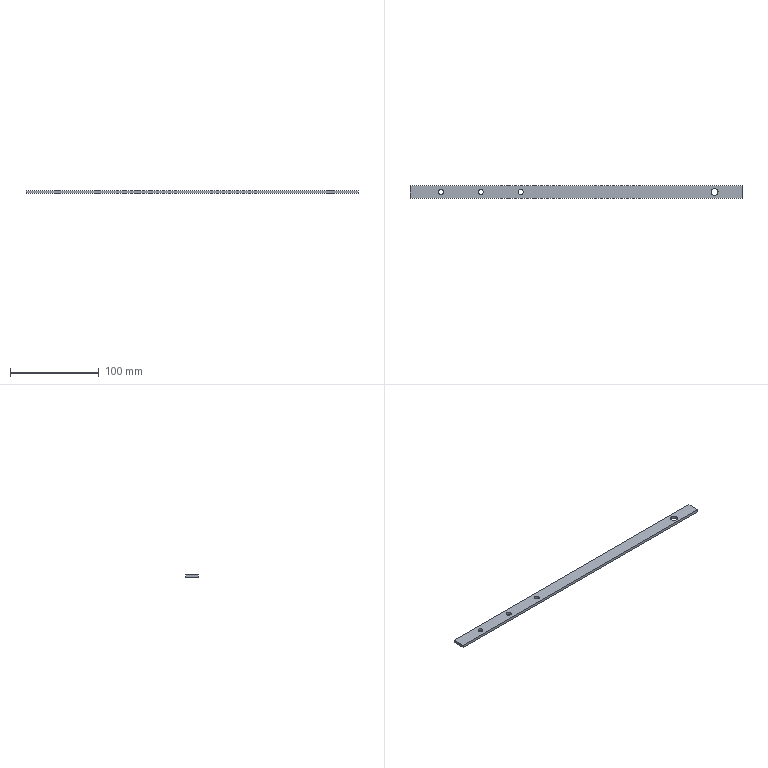Part | SolidWorks | features Extrusion 1, ICE 1 | 1 solid | 14 faces | box 375 x 14 x 3 mm | volume 15385 mm3 | cylinder 8 | plane 6 | commonest cylinder face diameters 5.5 x6 8 x2
STEP:
#1=CARTESIAN_POINT('',(152.5,0.,-1.5));
#2=VERTEX_POINT('',#1);
#3=CARTESIAN_POINT('',(160.5,0.,-1.5));
#4=VERTEX_POINT('',#3);
#5=CARTESIAN_POINT('',(156.5,0.,-1.5));
#6=DIRECTION('',(0.,0.,1.));
#7=DIRECTION('',(1.,0.,0.));
#8=AXIS2_PLACEMENT_3D('',#5,#6,#7);
#9=CIRCLE('',#8,4.);
#10=EDGE_CURVE('',#2,#4,#9,.T.);
#11=ORIENTED_EDGE('',*,*,#10,.F.);
#12=CARTESIAN_POINT('',(152.5,0.,1.5));
#13=VERTEX_POINT('',#12);
#14=CARTESIAN_POINT('',(152.5,0.,-1.5));
#15=DIRECTION('',(0.,0.,1.));
#16=VECTOR('',#15,1000.);
#17=LINE('',#14,#16);
#18=EDGE_CURVE('',#2,#13,#17,.T.);
#19=ORIENTED_EDGE('',*,*,#18,.T.);
#20=CARTESIAN_POINT('',(160.5,0.,1.5));
#21=VERTEX_POINT('',#20);
#22=CARTESIAN_POINT('',(156.5,0.,1.5));
#23=DIRECTION('',(0.,0.,1.));
#24=DIRECTION('',(1.,0.,0.));
#25=AXIS2_PLACEMENT_3D('',#22,#23,#24);
#26=CIRCLE('',#25,4.);
#27=EDGE_CURVE('',#13,#21,#26,.T.);
#28=ORIENTED_EDGE('',*,*,#27,.T.);
#29=CARTESIAN_POINT('',(160.5,0.,-1.5));
#30=DIRECTION('',(0.,0.,1.));
#31=VECTOR('',#30,1000.);
#32=LINE('',#29,#31);
#33=EDGE_CURVE('',#4,#21,#32,.T.);
#34=ORIENTED_EDGE('',*,*,#33,.F.);
#35=EDGE_LOOP('',(#11,#19,#28,#34));
#36=FACE_OUTER_BOUND('',#35,.T.);
#37=CARTESIAN_POINT('',(156.5,0.,-1.5));
#38=DIRECTION('',(0.,0.,1.));
#39=DIRECTION('',(1.,0.,0.));
#40=AXIS2_PLACEMENT_3D('',#37,#38,#39);
#41=CYLINDRICAL_SURFACE('',#40,4.);
#42=ADVANCED_FACE('',(#36),#41,.F.);
#43=CARTESIAN_POINT('',(-65.25,0.,1.5));
#44=VERTEX_POINT('',#43);
#45=CARTESIAN_POINT('',(-59.75,0.,1.5));
#46=VERTEX_POINT('',#45);
#47=CARTESIAN_POINT('',(-62.5,0.,1.5));
#48=DIRECTION('',(0.,0.,1.));
#49=DIRECTION('',(1.,0.,0.));
#50=AXIS2_PLACEMENT_3D('',#47,#48,#49);
#51=CIRCLE('',#50,2.75);
#52=EDGE_CURVE('',#44,#46,#51,.T.);
#53=ORIENTED_EDGE('',*,*,#52,.T.);
#54=CARTESIAN_POINT('',(-59.75,0.,-1.5));
#55=VERTEX_POINT('',#54);
#56=CARTESIAN_POINT('',(-59.75,0.,1.5));
#57=DIRECTION('',(0.,0.,-1.));
#58=VECTOR('',#57,1000.);
#59=LINE('',#56,#58);
#60=EDGE_CURVE('',#46,#55,#59,.T.);
#61=ORIENTED_EDGE('',*,*,#60,.T.);
#62=CARTESIAN_POINT('',(-65.25,0.,-1.5));
#63=VERTEX_POINT('',#62);
#64=CARTESIAN_POINT('',(-62.5,0.,-1.5));
#65=DIRECTION('',(0.,0.,1.));
#66=DIRECTION('',(1.,0.,0.));
#67=AXIS2_PLACEMENT_3D('',#64,#65,#66);
#68=CIRCLE('',#67,2.75);
#69=EDGE_CURVE('',#63,#55,#68,.T.);
#70=ORIENTED_EDGE('',*,*,#69,.F.);
#71=CARTESIAN_POINT('',(-65.25,0.,1.5));
#72=DIRECTION('',(0.,0.,-1.));
#73=VECTOR('',#72,1000.);
#74=LINE('',#71,#73);
#75=EDGE_CURVE('',#44,#63,#74,.T.);
#76=ORIENTED_EDGE('',*,*,#75,.F.);
#77=EDGE_LOOP('',(#53,#61,#70,#76));
#78=FACE_OUTER_BOUND('',#77,.T.);
#79=CARTESIAN_POINT('',(-62.5,0.,1.5));
#80=DIRECTION('',(0.,0.,-1.));
#81=DIRECTION('',(-1.,0.,0.));
#82=AXIS2_PLACEMENT_3D('',#79,#80,#81);
#83=CYLINDRICAL_SURFACE('',#82,2.75);
#84=ADVANCED_FACE('',(#78),#83,.F.);
#85=CARTESIAN_POINT('',(-110.25,0.,1.5));
#86=VERTEX_POINT('',#85);
#87=CARTESIAN_POINT('',(-104.75,0.,1.5));
#88=VERTEX_POINT('',#87);
#89=CARTESIAN_POINT('',(-107.5,0.,1.5));
#90=DIRECTION('',(0.,0.,1.));
#91=DIRECTION('',(1.,0.,0.));
#92=AXIS2_PLACEMENT_3D('',#89,#90,#91);
#93=CIRCLE('',#92,2.75);
#94=EDGE_CURVE('',#86,#88,#93,.T.);
#95=ORIENTED_EDGE('',*,*,#94,.T.);
#96=CARTESIAN_POINT('',(-104.75,0.,-1.5));
#97=VERTEX_POINT('',#96);
#98=CARTESIAN_POINT('',(-104.75,0.,1.5));
#99=DIRECTION('',(0.,0.,-1.));
#100=VECTOR('',#99,1000.);
#101=LINE('',#98,#100);
#102=EDGE_CURVE('',#88,#97,#101,.T.);
#103=ORIENTED_EDGE('',*,*,#102,.T.);
#104=CARTESIAN_POINT('',(-110.25,0.,-1.5));
#105=VERTEX_POINT('',#104);
#106=CARTESIAN_POINT('',(-107.5,0.,-1.5));
#107=DIRECTION('',(0.,0.,1.));
#108=DIRECTION('',(1.,0.,0.));
#109=AXIS2_PLACEMENT_3D('',#106,#107,#108);
#110=CIRCLE('',#109,2.75);
#111=EDGE_CURVE('',#105,#97,#110,.T.);
#112=ORIENTED_EDGE('',*,*,#111,.F.);
#113=CARTESIAN_POINT('',(-110.25,0.,1.5));
#114=DIRECTION('',(0.,0.,-1.));
#115=VECTOR('',#114,1000.);
#116=LINE('',#113,#115);
#117=EDGE_CURVE('',#86,#105,#116,.T.);
#118=ORIENTED_EDGE('',*,*,#117,.F.);
#119=EDGE_LOOP('',(#95,#103,#112,#118));
#120=FACE_OUTER_BOUND('',#119,.T.);
#121=CARTESIAN_POINT('',(-107.5,0.,1.5));
#122=DIRECTION('',(0.,0.,-1.));
#123=DIRECTION('',(-1.,0.,0.));
#124=AXIS2_PLACEMENT_3D('',#121,#122,#123);
#125=CYLINDRICAL_SURFACE('',#124,2.75);
#126=ADVANCED_FACE('',(#120),#125,.F.);
#127=CARTESIAN_POINT('',(-155.25,0.,1.5));
#128=VERTEX_POINT('',#127);
#129=CARTESIAN_POINT('',(-149.75,0.,1.5));
#130=VERTEX_POINT('',#129);
#131=CARTESIAN_POINT('',(-152.5,0.,1.5));
#132=DIRECTION('',(0.,0.,1.));
#133=DIRECTION('',(1.,0.,0.));
#134=AXIS2_PLACEMENT_3D('',#131,#132,#133);
#135=CIRCLE('',#134,2.75);
#136=EDGE_CURVE('',#128,#130,#135,.T.);
#137=ORIENTED_EDGE('',*,*,#136,.T.);
#138=CARTESIAN_POINT('',(-149.75,0.,-1.5));
#139=VERTEX_POINT('',#138);
#140=CARTESIAN_POINT('',(-149.75,0.,1.5));
#141=DIRECTION('',(0.,0.,-1.));
#142=VECTOR('',#141,1000.);
#143=LINE('',#140,#142);
#144=EDGE_CURVE('',#130,#139,#143,.T.);
#145=ORIENTED_EDGE('',*,*,#144,.T.);
#146=CARTESIAN_POINT('',(-155.25,0.,-1.5));
#147=VERTEX_POINT('',#146);
#148=CARTESIAN_POINT('',(-152.5,0.,-1.5));
#149=DIRECTION('',(0.,0.,1.));
#150=DIRECTION('',(1.,0.,0.));
#151=AXIS2_PLACEMENT_3D('',#148,#149,#150);
#152=CIRCLE('',#151,2.75);
#153=EDGE_CURVE('',#147,#139,#152,.T.);
#154=ORIENTED_EDGE('',*,*,#153,.F.);
#155=CARTESIAN_POINT('',(-155.25,0.,1.5));
#156=DIRECTION('',(0.,0.,-1.));
#157=VECTOR('',#156,1000.);
#158=LINE('',#155,#157);
#159=EDGE_CURVE('',#128,#147,#158,.T.);
#160=ORIENTED_EDGE('',*,*,#159,.F.);
#161=EDGE_LOOP('',(#137,#145,#154,#160));
#162=FACE_OUTER_BOUND('',#161,.T.);
#163=CARTESIAN_POINT('',(-152.5,0.,1.5));
#164=DIRECTION('',(0.,0.,-1.));
#165=DIRECTION('',(-1.,0.,0.));
#166=AXIS2_PLACEMENT_3D('',#163,#164,#165);
#167=CYLINDRICAL_SURFACE('',#166,2.75);
#168=ADVANCED_FACE('',(#162),#167,.F.);
#169=CARTESIAN_POINT('',(156.5,0.,1.5));
#170=DIRECTION('',(0.,0.,1.));
#171=DIRECTION('',(1.,0.,0.));
#172=AXIS2_PLACEMENT_3D('',#169,#170,#171);
#173=CIRCLE('',#172,4.);
#174=EDGE_CURVE('',#21,#13,#173,.T.);
#175=ORIENTED_EDGE('',*,*,#174,.F.);
#176=ORIENTED_EDGE('',*,*,#27,.F.);
#177=EDGE_LOOP('',(#175,#176));
#178=FACE_BOUND('',#177,.T.);
#179=ORIENTED_EDGE('',*,*,#94,.F.);
#180=CARTESIAN_POINT('',(-107.5,0.,1.5));
#181=DIRECTION('',(0.,0.,1.));
#182=DIRECTION('',(1.,0.,0.));
#183=AXIS2_PLACEMENT_3D('',#180,#181,#182);
#184=CIRCLE('',#183,2.75);
#185=EDGE_CURVE('',#88,#86,#184,.T.);
#186=ORIENTED_EDGE('',*,*,#185,.F.);
#187=EDGE_LOOP('',(#179,#186));
#188=FACE_BOUND('',#187,.T.);
#189=CARTESIAN_POINT('',(-187.5,7.,1.5));
#190=VERTEX_POINT('',#189);
#191=CARTESIAN_POINT('',(-187.5,-7.,1.5));
#192=VERTEX_POINT('',#191);
#193=CARTESIAN_POINT('',(-187.5,-7.,1.5));
#194=DIRECTION('',(0.,-1.,0.));
#195=VECTOR('',#194,1000.);
#196=LINE('',#193,#195);
#197=EDGE_CURVE('',#190,#192,#196,.T.);
#198=ORIENTED_EDGE('',*,*,#197,.T.);
#199=CARTESIAN_POINT('',(187.5,-7.,1.5));
#200=VERTEX_POINT('',#199);
#201=CARTESIAN_POINT('',(187.5,-7.,1.5));
#202=DIRECTION('',(1.,0.,0.));
#203=VECTOR('',#202,1000.);
#204=LINE('',#201,#203);
#205=EDGE_CURVE('',#192,#200,#204,.T.);
#206=ORIENTED_EDGE('',*,*,#205,.T.);
#207=CARTESIAN_POINT('',(187.5,7.,1.5));
#208=VERTEX_POINT('',#207);
#209=CARTESIAN_POINT('',(187.5,-7.,1.5));
#210=DIRECTION('',(0.,1.,0.));
#211=VECTOR('',#210,1000.);
#212=LINE('',#209,#211);
#213=EDGE_CURVE('',#200,#208,#212,.T.);
#214=ORIENTED_EDGE('',*,*,#213,.T.);
#215=CARTESIAN_POINT('',(187.5,7.,1.5));
#216=DIRECTION('',(-1.,0.,0.));
#217=VECTOR('',#216,1000.);
#218=LINE('',#215,#217);
#219=EDGE_CURVE('',#208,#190,#218,.T.);
#220=ORIENTED_EDGE('',*,*,#219,.T.);
#221=EDGE_LOOP('',(#198,#206,#214,#220));
#222=FACE_OUTER_BOUND('',#221,.T.);
#223=ORIENTED_EDGE('',*,*,#136,.F.);
#224=CARTESIAN_POINT('',(-152.5,0.,1.5));
#225=DIRECTION('',(0.,0.,1.));
#226=DIRECTION('',(1.,0.,0.));
#227=AXIS2_PLACEMENT_3D('',#224,#225,#226);
#228=CIRCLE('',#227,2.75);
#229=EDGE_CURVE('',#130,#128,#228,.T.);
#230=ORIENTED_EDGE('',*,*,#229,.F.);
#231=EDGE_LOOP('',(#223,#230));
#232=FACE_BOUND('',#231,.T.);
#233=ORIENTED_EDGE('',*,*,#52,.F.);
#234=CARTESIAN_POINT('',(-62.5,0.,1.5));
#235=DIRECTION('',(0.,0.,1.));
#236=DIRECTION('',(1.,0.,0.));
#237=AXIS2_PLACEMENT_3D('',#234,#235,#236);
#238=CIRCLE('',#237,2.75);
#239=EDGE_CURVE('',#46,#44,#238,.T.);
#240=ORIENTED_EDGE('',*,*,#239,.F.);
#241=EDGE_LOOP('',(#233,#240));
#242=FACE_BOUND('',#241,.T.);
#243=CARTESIAN_POINT('',(0.,0.,1.5));
#244=DIRECTION('',(0.,0.,1.));
#245=DIRECTION('',(1.,0.,0.));
#246=AXIS2_PLACEMENT_3D('',#243,#244,#245);
#247=PLANE('',#246);
#248=ADVANCED_FACE('',(#178,#188,#222,#232,#242),#247,.T.);
#249=CARTESIAN_POINT('',(156.5,0.,-1.5));
#250=DIRECTION('',(0.,0.,1.));
#251=DIRECTION('',(1.,0.,0.));
#252=AXIS2_PLACEMENT_3D('',#249,#250,#251);
#253=CIRCLE('',#252,4.);
#254=EDGE_CURVE('',#4,#2,#253,.T.);
#255=ORIENTED_EDGE('',*,*,#254,.T.);
#256=ORIENTED_EDGE('',*,*,#10,.T.);
#257=EDGE_LOOP('',(#255,#256));
#258=FACE_BOUND('',#257,.T.);
#259=CARTESIAN_POINT('',(-187.5,7.,-1.5));
#260=VERTEX_POINT('',#259);
#261=CARTESIAN_POINT('',(-187.5,-7.,-1.5));
#262=VERTEX_POINT('',#261);
#263=CARTESIAN_POINT('',(-187.5,-7.,-1.5));
#264=DIRECTION('',(0.,-1.,0.));
#265=VECTOR('',#264,1000.);
#266=LINE('',#263,#265);
#267=EDGE_CURVE('',#260,#262,#266,.T.);
#268=ORIENTED_EDGE('',*,*,#267,.F.);
#269=CARTESIAN_POINT('',(187.5,7.,-1.5));
#270=VERTEX_POINT('',#269);
#271=CARTESIAN_POINT('',(187.5,7.,-1.5));
#272=DIRECTION('',(-1.,0.,0.));
#273=VECTOR('',#272,1000.);
#274=LINE('',#271,#273);
#275=EDGE_CURVE('',#270,#260,#274,.T.);
#276=ORIENTED_EDGE('',*,*,#275,.F.);
#277=CARTESIAN_POINT('',(187.5,-7.,-1.5));
#278=VERTEX_POINT('',#277);
#279=CARTESIAN_POINT('',(187.5,-7.,-1.5));
#280=DIRECTION('',(0.,1.,0.));
#281=VECTOR('',#280,1000.);
#282=LINE('',#279,#281);
#283=EDGE_CURVE('',#278,#270,#282,.T.);
#284=ORIENTED_EDGE('',*,*,#283,.F.);
#285=CARTESIAN_POINT('',(187.5,-7.,-1.5));
#286=DIRECTION('',(1.,0.,0.));
#287=VECTOR('',#286,1000.);
#288=LINE('',#285,#287);
#289=EDGE_CURVE('',#262,#278,#288,.T.);
#290=ORIENTED_EDGE('',*,*,#289,.F.);
#291=EDGE_LOOP('',(#268,#276,#284,#290));
#292=FACE_OUTER_BOUND('',#291,.T.);
#293=ORIENTED_EDGE('',*,*,#153,.T.);
#294=CARTESIAN_POINT('',(-152.5,0.,-1.5));
#295=DIRECTION('',(0.,0.,1.));
#296=DIRECTION('',(1.,0.,0.));
#297=AXIS2_PLACEMENT_3D('',#294,#295,#296);
#298=CIRCLE('',#297,2.75);
#299=EDGE_CURVE('',#139,#147,#298,.T.);
#300=ORIENTED_EDGE('',*,*,#299,.T.);
#301=EDGE_LOOP('',(#293,#300));
#302=FACE_BOUND('',#301,.T.);
#303=ORIENTED_EDGE('',*,*,#111,.T.);
#304=CARTESIAN_POINT('',(-107.5,0.,-1.5));
#305=DIRECTION('',(0.,0.,1.));
#306=DIRECTION('',(1.,0.,0.));
#307=AXIS2_PLACEMENT_3D('',#304,#305,#306);
#308=CIRCLE('',#307,2.75);
#309=EDGE_CURVE('',#97,#105,#308,.T.);
#310=ORIENTED_EDGE('',*,*,#309,.T.);
#311=EDGE_LOOP('',(#303,#310));
#312=FACE_BOUND('',#311,.T.);
#313=ORIENTED_EDGE('',*,*,#69,.T.);
#314=CARTESIAN_POINT('',(-62.5,0.,-1.5));
#315=DIRECTION('',(0.,0.,1.));
#316=DIRECTION('',(1.,0.,0.));
#317=AXIS2_PLACEMENT_3D('',#314,#315,#316);
#318=CIRCLE('',#317,2.75);
#319=EDGE_CURVE('',#55,#63,#318,.T.);
#320=ORIENTED_EDGE('',*,*,#319,.T.);
#321=EDGE_LOOP('',(#313,#320));
#322=FACE_BOUND('',#321,.T.);
#323=CARTESIAN_POINT('',(0.,0.,-1.5));
#324=DIRECTION('',(0.,0.,1.));
#325=DIRECTION('',(1.,0.,0.));
#326=AXIS2_PLACEMENT_3D('',#323,#324,#325);
#327=PLANE('',#326);
#328=ADVANCED_FACE('',(#258,#292,#302,#312,#322),#327,.F.);
#329=ORIENTED_EDGE('',*,*,#267,.T.);
#330=CARTESIAN_POINT('',(-187.5,-7.,1.5));
#331=DIRECTION('',(0.,0.,-1.));
#332=VECTOR('',#331,1000.);
#333=LINE('',#330,#332);
#334=EDGE_CURVE('',#192,#262,#333,.T.);
#335=ORIENTED_EDGE('',*,*,#334,.F.);
#336=ORIENTED_EDGE('',*,*,#197,.F.);
#337=CARTESIAN_POINT('',(-187.5,7.,1.5));
#338=DIRECTION('',(0.,0.,-1.));
#339=VECTOR('',#338,1000.);
#340=LINE('',#337,#339);
#341=EDGE_CURVE('',#190,#260,#340,.T.);
#342=ORIENTED_EDGE('',*,*,#341,.T.);
#343=EDGE_LOOP('',(#329,#335,#336,#342));
#344=FACE_OUTER_BOUND('',#343,.T.);
#345=CARTESIAN_POINT('',(-187.5,-7.,1.5));
#346=DIRECTION('',(1.,0.,0.));
#347=DIRECTION('',(0.,0.,-1.));
#348=AXIS2_PLACEMENT_3D('',#345,#346,#347);
#349=PLANE('',#348);
#350=ADVANCED_FACE('',(#344),#349,.F.);
#351=ORIENTED_EDGE('',*,*,#289,.T.);
#352=CARTESIAN_POINT('',(187.5,-7.,1.5));
#353=DIRECTION('',(0.,0.,-1.));
#354=VECTOR('',#353,1000.);
#355=LINE('',#352,#354);
#356=EDGE_CURVE('',#200,#278,#355,.T.);
#357=ORIENTED_EDGE('',*,*,#356,.F.);
#358=ORIENTED_EDGE('',*,*,#205,.F.);
#359=ORIENTED_EDGE('',*,*,#334,.T.);
#360=EDGE_LOOP('',(#351,#357,#358,#359));
#361=FACE_OUTER_BOUND('',#360,.T.);
#362=CARTESIAN_POINT('',(187.5,-7.,1.5));
#363=DIRECTION('',(0.,1.,0.));
#364=DIRECTION('',(-1.,0.,0.));
#365=AXIS2_PLACEMENT_3D('',#362,#363,#364);
#366=PLANE('',#365);
#367=ADVANCED_FACE('',(#361),#366,.F.);
#368=ORIENTED_EDGE('',*,*,#283,.T.);
#369=CARTESIAN_POINT('',(187.5,7.,1.5));
#370=DIRECTION('',(0.,0.,-1.));
#371=VECTOR('',#370,1000.);
#372=LINE('',#369,#371);
#373=EDGE_CURVE('',#208,#270,#372,.T.);
#374=ORIENTED_EDGE('',*,*,#373,.F.);
#375=ORIENTED_EDGE('',*,*,#213,.F.);
#376=ORIENTED_EDGE('',*,*,#356,.T.);
#377=EDGE_LOOP('',(#368,#374,#375,#376));
#378=FACE_OUTER_BOUND('',#377,.T.);
#379=CARTESIAN_POINT('',(187.5,-7.,1.5));
#380=DIRECTION('',(-1.,0.,0.));
#381=DIRECTION('',(0.,0.,1.));
#382=AXIS2_PLACEMENT_3D('',#379,#380,#381);
#383=PLANE('',#382);
#384=ADVANCED_FACE('',(#378),#383,.F.);
#385=ORIENTED_EDGE('',*,*,#275,.T.);
#386=ORIENTED_EDGE('',*,*,#341,.F.);
#387=ORIENTED_EDGE('',*,*,#219,.F.);
#388=ORIENTED_EDGE('',*,*,#373,.T.);
#389=EDGE_LOOP('',(#385,#386,#387,#388));
#390=FACE_OUTER_BOUND('',#389,.T.);
#391=CARTESIAN_POINT('',(187.5,7.,1.5));
#392=DIRECTION('',(0.,-1.,0.));
#393=DIRECTION('',(1.,0.,0.));
#394=AXIS2_PLACEMENT_3D('',#391,#392,#393);
#395=PLANE('',#394);
#396=ADVANCED_FACE('',(#390),#395,.F.);
#397=ORIENTED_EDGE('',*,*,#144,.F.);
#398=ORIENTED_EDGE('',*,*,#229,.T.);
#399=ORIENTED_EDGE('',*,*,#159,.T.);
#400=ORIENTED_EDGE('',*,*,#299,.F.);
#401=EDGE_LOOP('',(#397,#398,#399,#400));
#402=FACE_OUTER_BOUND('',#401,.T.);
#403=CARTESIAN_POINT('',(-152.5,0.,1.5));
#404=DIRECTION('',(0.,0.,-1.));
#405=DIRECTION('',(-1.,0.,0.));
#406=AXIS2_PLACEMENT_3D('',#403,#404,#405);
#407=CYLINDRICAL_SURFACE('',#406,2.75);
#408=ADVANCED_FACE('',(#402),#407,.F.);
#409=ORIENTED_EDGE('',*,*,#102,.F.);
#410=ORIENTED_EDGE('',*,*,#185,.T.);
#411=ORIENTED_EDGE('',*,*,#117,.T.);
#412=ORIENTED_EDGE('',*,*,#309,.F.);
#413=EDGE_LOOP('',(#409,#410,#411,#412));
#414=FACE_OUTER_BOUND('',#413,.T.);
#415=CARTESIAN_POINT('',(-107.5,0.,1.5));
#416=DIRECTION('',(0.,0.,-1.));
#417=DIRECTION('',(-1.,0.,0.));
#418=AXIS2_PLACEMENT_3D('',#415,#416,#417);
#419=CYLINDRICAL_SURFACE('',#418,2.75);
#420=ADVANCED_FACE('',(#414),#419,.F.);
#421=ORIENTED_EDGE('',*,*,#60,.F.);
#422=ORIENTED_EDGE('',*,*,#239,.T.);
#423=ORIENTED_EDGE('',*,*,#75,.T.);
#424=ORIENTED_EDGE('',*,*,#319,.F.);
#425=EDGE_LOOP('',(#421,#422,#423,#424));
#426=FACE_OUTER_BOUND('',#425,.T.);
#427=CARTESIAN_POINT('',(-62.5,0.,1.5));
#428=DIRECTION('',(0.,0.,-1.));
#429=DIRECTION('',(-1.,0.,0.));
#430=AXIS2_PLACEMENT_3D('',#427,#428,#429);
#431=CYLINDRICAL_SURFACE('',#430,2.75);
#432=ADVANCED_FACE('',(#426),#431,.F.);
#433=ORIENTED_EDGE('',*,*,#18,.F.);
#434=ORIENTED_EDGE('',*,*,#254,.F.);
#435=ORIENTED_EDGE('',*,*,#33,.T.);
#436=ORIENTED_EDGE('',*,*,#174,.T.);
#437=EDGE_LOOP('',(#433,#434,#435,#436));
#438=FACE_OUTER_BOUND('',#437,.T.);
#439=CARTESIAN_POINT('',(156.5,0.,-1.5));
#440=DIRECTION('',(0.,0.,1.));
#441=DIRECTION('',(1.,0.,0.));
#442=AXIS2_PLACEMENT_3D('',#439,#440,#441);
#443=CYLINDRICAL_SURFACE('',#442,4.);
#444=ADVANCED_FACE('',(#438),#443,.F.);
#445=CLOSED_SHELL('',(#42,#84,#126,#168,#248,#328,#350,#367,#384,#396,#408,#420,#432,#444));
#446=MANIFOLD_SOLID_BREP('',#445);
#447=CARTESIAN_POINT('',(0.,0.,0.));
#448=DIRECTION('',(0.,0.,1.));
#449=DIRECTION('',(1.,0.,0.));
#450=AXIS2_PLACEMENT_3D('',#447,#448,#449);
#451=(LENGTH_UNIT()NAMED_UNIT(*)SI_UNIT(.MILLI.,.METRE.));
#452=UNCERTAINTY_MEASURE_WITH_UNIT(LENGTH_MEASURE(0.00001),#451,'','');
#453=(NAMED_UNIT(*)PLANE_ANGLE_UNIT()SI_UNIT($,.RADIAN.));
#454=(NAMED_UNIT(*)SI_UNIT($,.STERADIAN.)SOLID_ANGLE_UNIT());
#455=(GEOMETRIC_REPRESENTATION_CONTEXT(3)GLOBAL_UNCERTAINTY_ASSIGNED_CONTEXT((#452))GLOBAL_UNIT_ASSIGNED_CONTEXT((#451,#453,#454))REPRESENTATION_CONTEXT('',''));
#456=ADVANCED_BREP_SHAPE_REPRESENTATION('',(#446,#450),#455);